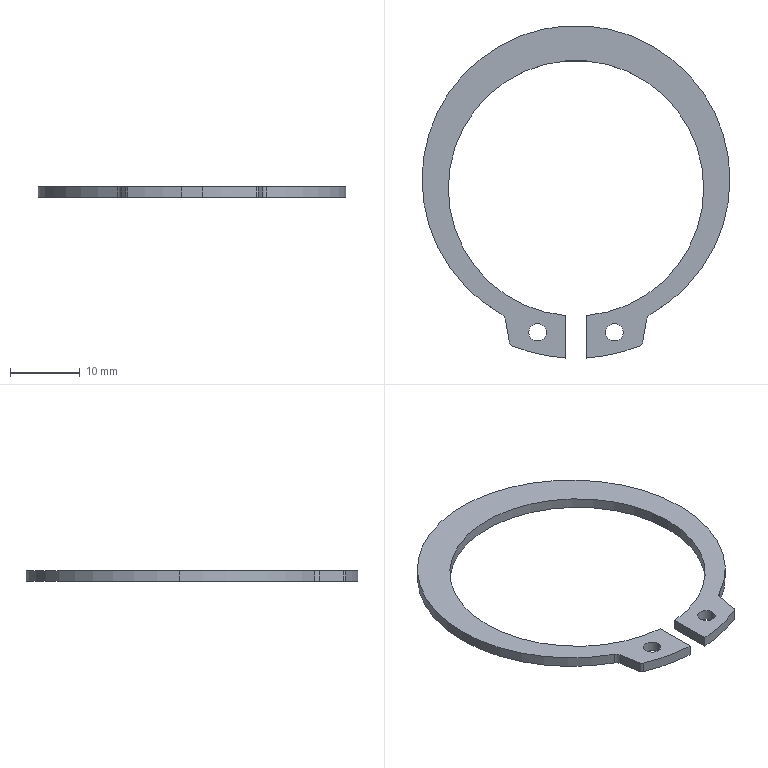Part | SolidWorks | features Extrusion 1 | 1 solid | 22 faces | box 44 x 47.504 x 1.5 mm | volume 776.12 mm3 | cylinder 16 | plane 6 | commonest cylinder face diameters 2.5 x4 36.5 x3 44 x3 1 x2 2 x2 48.6 x2
STEP:
#1=CARTESIAN_POINT('',(4.25,-21.828,0.75));
#2=VERTEX_POINT('',#1);
#3=CARTESIAN_POINT('',(6.75,-21.828,0.75));
#4=VERTEX_POINT('',#3);
#5=CARTESIAN_POINT('',(5.5,-21.828,0.75));
#6=DIRECTION('',(0.,0.,1.));
#7=DIRECTION('',(-1.,0.,0.));
#8=AXIS2_PLACEMENT_3D('',#5,#6,#7);
#9=CIRCLE('',#8,1.25);
#10=EDGE_CURVE('',#2,#4,#9,.T.);
#11=ORIENTED_EDGE('',*,*,#10,.T.);
#12=CARTESIAN_POINT('',(6.75,-21.828,-0.75));
#13=VERTEX_POINT('',#12);
#14=CARTESIAN_POINT('',(6.75,-21.828,0.75));
#15=DIRECTION('',(0.,0.,-1.));
#16=VECTOR('',#15,1000.);
#17=LINE('',#14,#16);
#18=EDGE_CURVE('',#4,#13,#17,.T.);
#19=ORIENTED_EDGE('',*,*,#18,.T.);
#20=CARTESIAN_POINT('',(4.25,-21.828,-0.75));
#21=VERTEX_POINT('',#20);
#22=CARTESIAN_POINT('',(5.5,-21.828,-0.75));
#23=DIRECTION('',(0.,0.,1.));
#24=DIRECTION('',(-1.,0.,0.));
#25=AXIS2_PLACEMENT_3D('',#22,#23,#24);
#26=CIRCLE('',#25,1.25);
#27=EDGE_CURVE('',#21,#13,#26,.T.);
#28=ORIENTED_EDGE('',*,*,#27,.F.);
#29=CARTESIAN_POINT('',(4.25,-21.828,0.75));
#30=DIRECTION('',(0.,0.,-1.));
#31=VECTOR('',#30,1000.);
#32=LINE('',#29,#31);
#33=EDGE_CURVE('',#2,#21,#32,.T.);
#34=ORIENTED_EDGE('',*,*,#33,.F.);
#35=EDGE_LOOP('',(#11,#19,#28,#34));
#36=FACE_OUTER_BOUND('',#35,.T.);
#37=CARTESIAN_POINT('',(5.5,-21.828,0.75));
#38=DIRECTION('',(0.,0.,-1.));
#39=DIRECTION('',(-1.,0.,0.));
#40=AXIS2_PLACEMENT_3D('',#37,#38,#39);
#41=CYLINDRICAL_SURFACE('',#40,1.25);
#42=ADVANCED_FACE('',(#36),#41,.F.);
#43=CARTESIAN_POINT('',(-6.75,-21.828,0.75));
#44=VERTEX_POINT('',#43);
#45=CARTESIAN_POINT('',(-4.25,-21.828,0.75));
#46=VERTEX_POINT('',#45);
#47=CARTESIAN_POINT('',(-5.5,-21.828,0.75));
#48=DIRECTION('',(0.,0.,1.));
#49=DIRECTION('',(1.,0.,0.));
#50=AXIS2_PLACEMENT_3D('',#47,#48,#49);
#51=CIRCLE('',#50,1.25);
#52=EDGE_CURVE('',#44,#46,#51,.T.);
#53=ORIENTED_EDGE('',*,*,#52,.T.);
#54=CARTESIAN_POINT('',(-4.25,-21.828,-0.75));
#55=VERTEX_POINT('',#54);
#56=CARTESIAN_POINT('',(-4.25,-21.828,0.75));
#57=DIRECTION('',(0.,0.,-1.));
#58=VECTOR('',#57,1000.);
#59=LINE('',#56,#58);
#60=EDGE_CURVE('',#46,#55,#59,.T.);
#61=ORIENTED_EDGE('',*,*,#60,.T.);
#62=CARTESIAN_POINT('',(-6.75,-21.828,-0.75));
#63=VERTEX_POINT('',#62);
#64=CARTESIAN_POINT('',(-5.5,-21.828,-0.75));
#65=DIRECTION('',(0.,0.,1.));
#66=DIRECTION('',(1.,0.,0.));
#67=AXIS2_PLACEMENT_3D('',#64,#65,#66);
#68=CIRCLE('',#67,1.25);
#69=EDGE_CURVE('',#63,#55,#68,.T.);
#70=ORIENTED_EDGE('',*,*,#69,.F.);
#71=CARTESIAN_POINT('',(-6.75,-21.828,0.75));
#72=DIRECTION('',(0.,0.,-1.));
#73=VECTOR('',#72,1000.);
#74=LINE('',#71,#73);
#75=EDGE_CURVE('',#44,#63,#74,.T.);
#76=ORIENTED_EDGE('',*,*,#75,.F.);
#77=EDGE_LOOP('',(#53,#61,#70,#76));
#78=FACE_OUTER_BOUND('',#77,.T.);
#79=CARTESIAN_POINT('',(-5.5,-21.828,0.75));
#80=DIRECTION('',(0.,0.,-1.));
#81=DIRECTION('',(-1.,0.,0.));
#82=AXIS2_PLACEMENT_3D('',#79,#80,#81);
#83=CYLINDRICAL_SURFACE('',#82,1.25);
#84=ADVANCED_FACE('',(#78),#83,.F.);
#85=CARTESIAN_POINT('',(22.,0.,0.75));
#86=VERTEX_POINT('',#85);
#87=CARTESIAN_POINT('',(-22.,0.,0.75));
#88=VERTEX_POINT('',#87);
#89=CARTESIAN_POINT('',(0.,0.,0.75));
#90=DIRECTION('',(0.,0.,1.));
#91=DIRECTION('',(1.,0.,0.));
#92=AXIS2_PLACEMENT_3D('',#89,#90,#91);
#93=CIRCLE('',#92,22.);
#94=EDGE_CURVE('',#86,#88,#93,.T.);
#95=ORIENTED_EDGE('',*,*,#94,.F.);
#96=CARTESIAN_POINT('',(22.,0.,-0.75));
#97=VERTEX_POINT('',#96);
#98=CARTESIAN_POINT('',(22.,0.,0.75));
#99=DIRECTION('',(0.,0.,-1.));
#100=VECTOR('',#99,1000.);
#101=LINE('',#98,#100);
#102=EDGE_CURVE('',#86,#97,#101,.T.);
#103=ORIENTED_EDGE('',*,*,#102,.T.);
#104=CARTESIAN_POINT('',(-22.,0.,-0.75));
#105=VERTEX_POINT('',#104);
#106=CARTESIAN_POINT('',(0.,0.,-0.75));
#107=DIRECTION('',(0.,0.,1.));
#108=DIRECTION('',(1.,0.,0.));
#109=AXIS2_PLACEMENT_3D('',#106,#107,#108);
#110=CIRCLE('',#109,22.);
#111=EDGE_CURVE('',#97,#105,#110,.T.);
#112=ORIENTED_EDGE('',*,*,#111,.T.);
#113=CARTESIAN_POINT('',(-22.,0.,0.75));
#114=DIRECTION('',(0.,0.,-1.));
#115=VECTOR('',#114,1000.);
#116=LINE('',#113,#115);
#117=EDGE_CURVE('',#88,#105,#116,.T.);
#118=ORIENTED_EDGE('',*,*,#117,.F.);
#119=EDGE_LOOP('',(#95,#103,#112,#118));
#120=FACE_OUTER_BOUND('',#119,.T.);
#121=CARTESIAN_POINT('',(0.,0.,0.75));
#122=DIRECTION('',(0.,0.,-1.));
#123=DIRECTION('',(-1.,0.,0.));
#124=AXIS2_PLACEMENT_3D('',#121,#122,#123);
#125=CYLINDRICAL_SURFACE('',#124,22.);
#126=ADVANCED_FACE('',(#120),#125,.T.);
#127=CARTESIAN_POINT('',(-10.6,-19.278,0.75));
#128=VERTEX_POINT('',#127);
#129=CARTESIAN_POINT('',(0.,0.,0.75));
#130=DIRECTION('',(0.,0.,1.));
#131=DIRECTION('',(1.,0.,0.));
#132=AXIS2_PLACEMENT_3D('',#129,#130,#131);
#133=CIRCLE('',#132,22.);
#134=EDGE_CURVE('',#88,#128,#133,.T.);
#135=ORIENTED_EDGE('',*,*,#134,.F.);
#136=ORIENTED_EDGE('',*,*,#117,.T.);
#137=CARTESIAN_POINT('',(-10.6,-19.278,-0.75));
#138=VERTEX_POINT('',#137);
#139=CARTESIAN_POINT('',(0.,0.,-0.75));
#140=DIRECTION('',(0.,0.,1.));
#141=DIRECTION('',(1.,0.,0.));
#142=AXIS2_PLACEMENT_3D('',#139,#140,#141);
#143=CIRCLE('',#142,22.);
#144=EDGE_CURVE('',#105,#138,#143,.T.);
#145=ORIENTED_EDGE('',*,*,#144,.T.);
#146=CARTESIAN_POINT('',(-10.6,-19.278,0.75));
#147=DIRECTION('',(0.,0.,-1.));
#148=VECTOR('',#147,1000.);
#149=LINE('',#146,#148);
#150=EDGE_CURVE('',#128,#138,#149,.T.);
#151=ORIENTED_EDGE('',*,*,#150,.F.);
#152=EDGE_LOOP('',(#135,#136,#145,#151));
#153=FACE_OUTER_BOUND('',#152,.T.);
#154=CARTESIAN_POINT('',(0.,0.,0.75));
#155=DIRECTION('',(0.,0.,-1.));
#156=DIRECTION('',(-1.,0.,0.));
#157=AXIS2_PLACEMENT_3D('',#154,#155,#156);
#158=CYLINDRICAL_SURFACE('',#157,22.);
#159=ADVANCED_FACE('',(#153),#158,.T.);
#160=CARTESIAN_POINT('',(18.25,-1.25,0.75));
#161=VERTEX_POINT('',#160);
#162=CARTESIAN_POINT('',(1.5,-19.438,0.75));
#163=VERTEX_POINT('',#162);
#164=CARTESIAN_POINT('',(0.,-1.25,0.75));
#165=DIRECTION('',(0.,0.,-1.));
#166=DIRECTION('',(1.,0.,0.));
#167=AXIS2_PLACEMENT_3D('',#164,#165,#166);
#168=CIRCLE('',#167,18.25);
#169=EDGE_CURVE('',#161,#163,#168,.T.);
#170=ORIENTED_EDGE('',*,*,#169,.F.);
#171=CARTESIAN_POINT('',(18.25,-1.25,-0.75));
#172=VERTEX_POINT('',#171);
#173=CARTESIAN_POINT('',(18.25,-1.25,0.75));
#174=DIRECTION('',(0.,0.,-1.));
#175=VECTOR('',#174,1000.);
#176=LINE('',#173,#175);
#177=EDGE_CURVE('',#161,#172,#176,.T.);
#178=ORIENTED_EDGE('',*,*,#177,.T.);
#179=CARTESIAN_POINT('',(1.5,-19.438,-0.75));
#180=VERTEX_POINT('',#179);
#181=CARTESIAN_POINT('',(0.,-1.25,-0.75));
#182=DIRECTION('',(0.,0.,-1.));
#183=DIRECTION('',(1.,0.,0.));
#184=AXIS2_PLACEMENT_3D('',#181,#182,#183);
#185=CIRCLE('',#184,18.25);
#186=EDGE_CURVE('',#172,#180,#185,.T.);
#187=ORIENTED_EDGE('',*,*,#186,.T.);
#188=CARTESIAN_POINT('',(1.5,-19.438,0.75));
#189=DIRECTION('',(0.,0.,-1.));
#190=VECTOR('',#189,1000.);
#191=LINE('',#188,#190);
#192=EDGE_CURVE('',#163,#180,#191,.T.);
#193=ORIENTED_EDGE('',*,*,#192,.F.);
#194=EDGE_LOOP('',(#170,#178,#187,#193));
#195=FACE_OUTER_BOUND('',#194,.T.);
#196=CARTESIAN_POINT('',(0.,-1.25,0.75));
#197=DIRECTION('',(0.,0.,-1.));
#198=DIRECTION('',(-1.,0.,0.));
#199=AXIS2_PLACEMENT_3D('',#196,#197,#198);
#200=CYLINDRICAL_SURFACE('',#199,18.25);
#201=ADVANCED_FACE('',(#195),#200,.F.);
#202=ORIENTED_EDGE('',*,*,#177,.F.);
#203=CARTESIAN_POINT('',(-18.25,-1.25,0.75));
#204=VERTEX_POINT('',#203);
#205=CARTESIAN_POINT('',(0.,-1.25,0.75));
#206=DIRECTION('',(0.,0.,-1.));
#207=DIRECTION('',(1.,0.,0.));
#208=AXIS2_PLACEMENT_3D('',#205,#206,#207);
#209=CIRCLE('',#208,18.25);
#210=EDGE_CURVE('',#204,#161,#209,.T.);
#211=ORIENTED_EDGE('',*,*,#210,.F.);
#212=CARTESIAN_POINT('',(-18.25,-1.25,-0.75));
#213=VERTEX_POINT('',#212);
#214=CARTESIAN_POINT('',(-18.25,-1.25,0.75));
#215=DIRECTION('',(0.,0.,-1.));
#216=VECTOR('',#215,1000.);
#217=LINE('',#214,#216);
#218=EDGE_CURVE('',#204,#213,#217,.T.);
#219=ORIENTED_EDGE('',*,*,#218,.T.);
#220=CARTESIAN_POINT('',(0.,-1.25,-0.75));
#221=DIRECTION('',(0.,0.,-1.));
#222=DIRECTION('',(1.,0.,0.));
#223=AXIS2_PLACEMENT_3D('',#220,#221,#222);
#224=CIRCLE('',#223,18.25);
#225=EDGE_CURVE('',#213,#172,#224,.T.);
#226=ORIENTED_EDGE('',*,*,#225,.T.);
#227=EDGE_LOOP('',(#202,#211,#219,#226));
#228=FACE_OUTER_BOUND('',#227,.T.);
#229=CARTESIAN_POINT('',(0.,-1.25,0.75));
#230=DIRECTION('',(0.,0.,-1.));
#231=DIRECTION('',(-1.,0.,0.));
#232=AXIS2_PLACEMENT_3D('',#229,#230,#231);
#233=CYLINDRICAL_SURFACE('',#232,18.25);
#234=ADVANCED_FACE('',(#228),#233,.F.);
#235=ORIENTED_EDGE('',*,*,#52,.F.);
#236=CARTESIAN_POINT('',(-5.5,-21.828,0.75));
#237=DIRECTION('',(0.,0.,1.));
#238=DIRECTION('',(1.,0.,0.));
#239=AXIS2_PLACEMENT_3D('',#236,#237,#238);
#240=CIRCLE('',#239,1.25);
#241=EDGE_CURVE('',#46,#44,#240,.T.);
#242=ORIENTED_EDGE('',*,*,#241,.F.);
#243=EDGE_LOOP('',(#235,#242));
#244=FACE_BOUND('',#243,.T.);
#245=CARTESIAN_POINT('',(-10.097,-19.981,0.75));
#246=VERTEX_POINT('',#245);
#247=CARTESIAN_POINT('',(-11.082,-20.154,0.75));
#248=DIRECTION('',(0.,0.,-1.));
#249=DIRECTION('',(1.,0.,0.));
#250=AXIS2_PLACEMENT_3D('',#247,#248,#249);
#251=CIRCLE('',#250,1.);
#252=EDGE_CURVE('',#128,#246,#251,.T.);
#253=ORIENTED_EDGE('',*,*,#252,.T.);
#254=CARTESIAN_POINT('',(-9.5,-23.366,0.75));
#255=VERTEX_POINT('',#254);
#256=CARTESIAN_POINT('',(-10.097,-19.981,0.75));
#257=DIRECTION('',(0.1736,-0.9848,0.));
#258=VECTOR('',#257,1000.);
#259=LINE('',#256,#258);
#260=EDGE_CURVE('',#246,#255,#259,.T.);
#261=ORIENTED_EDGE('',*,*,#260,.T.);
#262=CARTESIAN_POINT('',(-9.197,-23.742,0.75));
#263=VERTEX_POINT('',#262);
#264=CARTESIAN_POINT('',(-9.008,-23.28,0.75));
#265=DIRECTION('',(0.,0.,1.));
#266=DIRECTION('',(-1.,0.,0.));
#267=AXIS2_PLACEMENT_3D('',#264,#265,#266);
#268=CIRCLE('',#267,0.5);
#269=EDGE_CURVE('',#255,#263,#268,.T.);
#270=ORIENTED_EDGE('',*,*,#269,.T.);
#271=CARTESIAN_POINT('',(-1.5,-25.504,0.75));
#272=VERTEX_POINT('',#271);
#273=CARTESIAN_POINT('',(0.,-1.25,0.75));
#274=DIRECTION('',(0.,0.,1.));
#275=DIRECTION('',(-1.,0.,0.));
#276=AXIS2_PLACEMENT_3D('',#273,#274,#275);
#277=CIRCLE('',#276,24.3);
#278=EDGE_CURVE('',#263,#272,#277,.T.);
#279=ORIENTED_EDGE('',*,*,#278,.T.);
#280=CARTESIAN_POINT('',(-1.5,-19.438,0.75));
#281=VERTEX_POINT('',#280);
#282=CARTESIAN_POINT('',(-1.5,-19.438,0.75));
#283=DIRECTION('',(0.,1.,0.));
#284=VECTOR('',#283,1000.);
#285=LINE('',#282,#284);
#286=EDGE_CURVE('',#272,#281,#285,.T.);
#287=ORIENTED_EDGE('',*,*,#286,.T.);
#288=CARTESIAN_POINT('',(0.,-1.25,0.75));
#289=DIRECTION('',(0.,0.,-1.));
#290=DIRECTION('',(1.,0.,0.));
#291=AXIS2_PLACEMENT_3D('',#288,#289,#290);
#292=CIRCLE('',#291,18.25);
#293=EDGE_CURVE('',#281,#204,#292,.T.);
#294=ORIENTED_EDGE('',*,*,#293,.T.);
#295=ORIENTED_EDGE('',*,*,#210,.T.);
#296=ORIENTED_EDGE('',*,*,#169,.T.);
#297=CARTESIAN_POINT('',(1.5,-25.504,0.75));
#298=VERTEX_POINT('',#297);
#299=CARTESIAN_POINT('',(1.5,-19.438,0.75));
#300=DIRECTION('',(0.,-1.,0.));
#301=VECTOR('',#300,1000.);
#302=LINE('',#299,#301);
#303=EDGE_CURVE('',#163,#298,#302,.T.);
#304=ORIENTED_EDGE('',*,*,#303,.T.);
#305=CARTESIAN_POINT('',(9.197,-23.742,0.75));
#306=VERTEX_POINT('',#305);
#307=CARTESIAN_POINT('',(0.,-1.25,0.75));
#308=DIRECTION('',(0.,0.,1.));
#309=DIRECTION('',(1.,0.,0.));
#310=AXIS2_PLACEMENT_3D('',#307,#308,#309);
#311=CIRCLE('',#310,24.3);
#312=EDGE_CURVE('',#298,#306,#311,.T.);
#313=ORIENTED_EDGE('',*,*,#312,.T.);
#314=CARTESIAN_POINT('',(9.5,-23.366,0.75));
#315=VERTEX_POINT('',#314);
#316=CARTESIAN_POINT('',(9.008,-23.28,0.75));
#317=DIRECTION('',(0.,0.,1.));
#318=DIRECTION('',(1.,0.,0.));
#319=AXIS2_PLACEMENT_3D('',#316,#317,#318);
#320=CIRCLE('',#319,0.5);
#321=EDGE_CURVE('',#306,#315,#320,.T.);
#322=ORIENTED_EDGE('',*,*,#321,.T.);
#323=CARTESIAN_POINT('',(10.097,-19.981,0.75));
#324=VERTEX_POINT('',#323);
#325=CARTESIAN_POINT('',(10.097,-19.981,0.75));
#326=DIRECTION('',(0.1736,0.9848,0.));
#327=VECTOR('',#326,1000.);
#328=LINE('',#325,#327);
#329=EDGE_CURVE('',#315,#324,#328,.T.);
#330=ORIENTED_EDGE('',*,*,#329,.T.);
#331=CARTESIAN_POINT('',(10.6,-19.278,0.75));
#332=VERTEX_POINT('',#331);
#333=CARTESIAN_POINT('',(11.082,-20.154,0.75));
#334=DIRECTION('',(0.,0.,-1.));
#335=DIRECTION('',(-1.,0.,0.));
#336=AXIS2_PLACEMENT_3D('',#333,#334,#335);
#337=CIRCLE('',#336,1.);
#338=EDGE_CURVE('',#324,#332,#337,.T.);
#339=ORIENTED_EDGE('',*,*,#338,.T.);
#340=CARTESIAN_POINT('',(0.,0.,0.75));
#341=DIRECTION('',(0.,0.,1.));
#342=DIRECTION('',(1.,0.,0.));
#343=AXIS2_PLACEMENT_3D('',#340,#341,#342);
#344=CIRCLE('',#343,22.);
#345=EDGE_CURVE('',#332,#86,#344,.T.);
#346=ORIENTED_EDGE('',*,*,#345,.T.);
#347=ORIENTED_EDGE('',*,*,#94,.T.);
#348=ORIENTED_EDGE('',*,*,#134,.T.);
#349=EDGE_LOOP('',(#253,#261,#270,#279,#287,#294,#295,#296,#304,#313,#322,#330,#339,#346,#347,#348));
#350=FACE_OUTER_BOUND('',#349,.T.);
#351=ORIENTED_EDGE('',*,*,#10,.F.);
#352=CARTESIAN_POINT('',(5.5,-21.828,0.75));
#353=DIRECTION('',(0.,0.,1.));
#354=DIRECTION('',(-1.,0.,0.));
#355=AXIS2_PLACEMENT_3D('',#352,#353,#354);
#356=CIRCLE('',#355,1.25);
#357=EDGE_CURVE('',#4,#2,#356,.T.);
#358=ORIENTED_EDGE('',*,*,#357,.F.);
#359=EDGE_LOOP('',(#351,#358));
#360=FACE_BOUND('',#359,.T.);
#361=CARTESIAN_POINT('',(-11.082,-20.154,0.75));
#362=DIRECTION('',(0.,0.,1.));
#363=DIRECTION('',(1.,0.,0.));
#364=AXIS2_PLACEMENT_3D('',#361,#362,#363);
#365=PLANE('',#364);
#366=ADVANCED_FACE('',(#244,#350,#360),#365,.T.);
#367=ORIENTED_EDGE('',*,*,#150,.T.);
#368=CARTESIAN_POINT('',(-10.097,-19.981,-0.75));
#369=VERTEX_POINT('',#368);
#370=CARTESIAN_POINT('',(-11.082,-20.154,-0.75));
#371=DIRECTION('',(0.,0.,-1.));
#372=DIRECTION('',(1.,0.,0.));
#373=AXIS2_PLACEMENT_3D('',#370,#371,#372);
#374=CIRCLE('',#373,1.);
#375=EDGE_CURVE('',#138,#369,#374,.T.);
#376=ORIENTED_EDGE('',*,*,#375,.T.);
#377=CARTESIAN_POINT('',(-10.097,-19.981,0.75));
#378=DIRECTION('',(0.,0.,-1.));
#379=VECTOR('',#378,1000.);
#380=LINE('',#377,#379);
#381=EDGE_CURVE('',#246,#369,#380,.T.);
#382=ORIENTED_EDGE('',*,*,#381,.F.);
#383=ORIENTED_EDGE('',*,*,#252,.F.);
#384=EDGE_LOOP('',(#367,#376,#382,#383));
#385=FACE_OUTER_BOUND('',#384,.T.);
#386=CARTESIAN_POINT('',(-11.082,-20.154,0.75));
#387=DIRECTION('',(0.,0.,-1.));
#388=DIRECTION('',(-1.,0.,0.));
#389=AXIS2_PLACEMENT_3D('',#386,#387,#388);
#390=CYLINDRICAL_SURFACE('',#389,1.);
#391=ADVANCED_FACE('',(#385),#390,.F.);
#392=ORIENTED_EDGE('',*,*,#381,.T.);
#393=CARTESIAN_POINT('',(-9.5,-23.366,-0.75));
#394=VERTEX_POINT('',#393);
#395=CARTESIAN_POINT('',(-10.097,-19.981,-0.75));
#396=DIRECTION('',(0.1736,-0.9848,0.));
#397=VECTOR('',#396,1000.);
#398=LINE('',#395,#397);
#399=EDGE_CURVE('',#369,#394,#398,.T.);
#400=ORIENTED_EDGE('',*,*,#399,.T.);
#401=CARTESIAN_POINT('',(-9.5,-23.366,0.75));
#402=DIRECTION('',(0.,0.,-1.));
#403=VECTOR('',#402,1000.);
#404=LINE('',#401,#403);
#405=EDGE_CURVE('',#255,#394,#404,.T.);
#406=ORIENTED_EDGE('',*,*,#405,.F.);
#407=ORIENTED_EDGE('',*,*,#260,.F.);
#408=EDGE_LOOP('',(#392,#400,#406,#407));
#409=FACE_OUTER_BOUND('',#408,.T.);
#410=CARTESIAN_POINT('',(-10.097,-19.981,0.75));
#411=DIRECTION('',(0.9848,0.1736,0.));
#412=DIRECTION('',(-0.1736,0.9848,0.));
#413=AXIS2_PLACEMENT_3D('',#410,#411,#412);
#414=PLANE('',#413);
#415=ADVANCED_FACE('',(#409),#414,.F.);
#416=ORIENTED_EDGE('',*,*,#405,.T.);
#417=CARTESIAN_POINT('',(-9.197,-23.742,-0.75));
#418=VERTEX_POINT('',#417);
#419=CARTESIAN_POINT('',(-9.008,-23.28,-0.75));
#420=DIRECTION('',(0.,0.,1.));
#421=DIRECTION('',(-1.,0.,0.));
#422=AXIS2_PLACEMENT_3D('',#419,#420,#421);
#423=CIRCLE('',#422,0.5);
#424=EDGE_CURVE('',#394,#418,#423,.T.);
#425=ORIENTED_EDGE('',*,*,#424,.T.);
#426=CARTESIAN_POINT('',(-9.197,-23.742,0.75));
#427=DIRECTION('',(0.,0.,-1.));
#428=VECTOR('',#427,1000.);
#429=LINE('',#426,#428);
#430=EDGE_CURVE('',#263,#418,#429,.T.);
#431=ORIENTED_EDGE('',*,*,#430,.F.);
#432=ORIENTED_EDGE('',*,*,#269,.F.);
#433=EDGE_LOOP('',(#416,#425,#431,#432));
#434=FACE_OUTER_BOUND('',#433,.T.);
#435=CARTESIAN_POINT('',(-9.008,-23.28,0.75));
#436=DIRECTION('',(0.,0.,-1.));
#437=DIRECTION('',(-1.,0.,0.));
#438=AXIS2_PLACEMENT_3D('',#435,#436,#437);
#439=CYLINDRICAL_SURFACE('',#438,0.5);
#440=ADVANCED_FACE('',(#434),#439,.T.);
#441=ORIENTED_EDGE('',*,*,#430,.T.);
#442=CARTESIAN_POINT('',(-1.5,-25.504,-0.75));
#443=VERTEX_POINT('',#442);
#444=CARTESIAN_POINT('',(0.,-1.25,-0.75));
#445=DIRECTION('',(0.,0.,1.));
#446=DIRECTION('',(-1.,0.,0.));
#447=AXIS2_PLACEMENT_3D('',#444,#445,#446);
#448=CIRCLE('',#447,24.3);
#449=EDGE_CURVE('',#418,#443,#448,.T.);
#450=ORIENTED_EDGE('',*,*,#449,.T.);
#451=CARTESIAN_POINT('',(-1.5,-25.504,0.75));
#452=DIRECTION('',(0.,0.,-1.));
#453=VECTOR('',#452,1000.);
#454=LINE('',#451,#453);
#455=EDGE_CURVE('',#272,#443,#454,.T.);
#456=ORIENTED_EDGE('',*,*,#455,.F.);
#457=ORIENTED_EDGE('',*,*,#278,.F.);
#458=EDGE_LOOP('',(#441,#450,#456,#457));
#459=FACE_OUTER_BOUND('',#458,.T.);
#460=CARTESIAN_POINT('',(0.,-1.25,0.75));
#461=DIRECTION('',(0.,0.,-1.));
#462=DIRECTION('',(-1.,0.,0.));
#463=AXIS2_PLACEMENT_3D('',#460,#461,#462);
#464=CYLINDRICAL_SURFACE('',#463,24.3);
#465=ADVANCED_FACE('',(#459),#464,.T.);
#466=ORIENTED_EDGE('',*,*,#455,.T.);
#467=CARTESIAN_POINT('',(-1.5,-19.438,-0.75));
#468=VERTEX_POINT('',#467);
#469=CARTESIAN_POINT('',(-1.5,-19.438,-0.75));
#470=DIRECTION('',(0.,1.,0.));
#471=VECTOR('',#470,1000.);
#472=LINE('',#469,#471);
#473=EDGE_CURVE('',#443,#468,#472,.T.);
#474=ORIENTED_EDGE('',*,*,#473,.T.);
#475=CARTESIAN_POINT('',(-1.5,-19.438,0.75));
#476=DIRECTION('',(0.,0.,-1.));
#477=VECTOR('',#476,1000.);
#478=LINE('',#475,#477);
#479=EDGE_CURVE('',#281,#468,#478,.T.);
#480=ORIENTED_EDGE('',*,*,#479,.F.);
#481=ORIENTED_EDGE('',*,*,#286,.F.);
#482=EDGE_LOOP('',(#466,#474,#480,#481));
#483=FACE_OUTER_BOUND('',#482,.T.);
#484=CARTESIAN_POINT('',(-1.5,-19.438,0.75));
#485=DIRECTION('',(-1.,0.,0.));
#486=DIRECTION('',(0.,-1.,0.));
#487=AXIS2_PLACEMENT_3D('',#484,#485,#486);
#488=PLANE('',#487);
#489=ADVANCED_FACE('',(#483),#488,.F.);
#490=ORIENTED_EDGE('',*,*,#218,.F.);
#491=ORIENTED_EDGE('',*,*,#293,.F.);
#492=ORIENTED_EDGE('',*,*,#479,.T.);
#493=CARTESIAN_POINT('',(0.,-1.25,-0.75));
#494=DIRECTION('',(0.,0.,-1.));
#495=DIRECTION('',(1.,0.,0.));
#496=AXIS2_PLACEMENT_3D('',#493,#494,#495);
#497=CIRCLE('',#496,18.25);
#498=EDGE_CURVE('',#468,#213,#497,.T.);
#499=ORIENTED_EDGE('',*,*,#498,.T.);
#500=EDGE_LOOP('',(#490,#491,#492,#499));
#501=FACE_OUTER_BOUND('',#500,.T.);
#502=CARTESIAN_POINT('',(0.,-1.25,0.75));
#503=DIRECTION('',(0.,0.,-1.));
#504=DIRECTION('',(-1.,0.,0.));
#505=AXIS2_PLACEMENT_3D('',#502,#503,#504);
#506=CYLINDRICAL_SURFACE('',#505,18.25);
#507=ADVANCED_FACE('',(#501),#506,.F.);
#508=ORIENTED_EDGE('',*,*,#192,.T.);
#509=CARTESIAN_POINT('',(1.5,-25.504,-0.75));
#510=VERTEX_POINT('',#509);
#511=CARTESIAN_POINT('',(1.5,-19.438,-0.75));
#512=DIRECTION('',(0.,-1.,0.));
#513=VECTOR('',#512,1000.);
#514=LINE('',#511,#513);
#515=EDGE_CURVE('',#180,#510,#514,.T.);
#516=ORIENTED_EDGE('',*,*,#515,.T.);
#517=CARTESIAN_POINT('',(1.5,-25.504,0.75));
#518=DIRECTION('',(0.,0.,-1.));
#519=VECTOR('',#518,1000.);
#520=LINE('',#517,#519);
#521=EDGE_CURVE('',#298,#510,#520,.T.);
#522=ORIENTED_EDGE('',*,*,#521,.F.);
#523=ORIENTED_EDGE('',*,*,#303,.F.);
#524=EDGE_LOOP('',(#508,#516,#522,#523));
#525=FACE_OUTER_BOUND('',#524,.T.);
#526=CARTESIAN_POINT('',(1.5,-19.438,0.75));
#527=DIRECTION('',(1.,0.,0.));
#528=DIRECTION('',(0.,1.,0.));
#529=AXIS2_PLACEMENT_3D('',#526,#527,#528);
#530=PLANE('',#529);
#531=ADVANCED_FACE('',(#525),#530,.F.);
#532=ORIENTED_EDGE('',*,*,#521,.T.);
#533=CARTESIAN_POINT('',(9.197,-23.742,-0.75));
#534=VERTEX_POINT('',#533);
#535=CARTESIAN_POINT('',(0.,-1.25,-0.75));
#536=DIRECTION('',(0.,0.,1.));
#537=DIRECTION('',(1.,0.,0.));
#538=AXIS2_PLACEMENT_3D('',#535,#536,#537);
#539=CIRCLE('',#538,24.3);
#540=EDGE_CURVE('',#510,#534,#539,.T.);
#541=ORIENTED_EDGE('',*,*,#540,.T.);
#542=CARTESIAN_POINT('',(9.197,-23.742,0.75));
#543=DIRECTION('',(0.,0.,-1.));
#544=VECTOR('',#543,1000.);
#545=LINE('',#542,#544);
#546=EDGE_CURVE('',#306,#534,#545,.T.);
#547=ORIENTED_EDGE('',*,*,#546,.F.);
#548=ORIENTED_EDGE('',*,*,#312,.F.);
#549=EDGE_LOOP('',(#532,#541,#547,#548));
#550=FACE_OUTER_BOUND('',#549,.T.);
#551=CARTESIAN_POINT('',(0.,-1.25,0.75));
#552=DIRECTION('',(0.,0.,-1.));
#553=DIRECTION('',(-1.,0.,0.));
#554=AXIS2_PLACEMENT_3D('',#551,#552,#553);
#555=CYLINDRICAL_SURFACE('',#554,24.3);
#556=ADVANCED_FACE('',(#550),#555,.T.);
#557=ORIENTED_EDGE('',*,*,#546,.T.);
#558=CARTESIAN_POINT('',(9.5,-23.366,-0.75));
#559=VERTEX_POINT('',#558);
#560=CARTESIAN_POINT('',(9.008,-23.28,-0.75));
#561=DIRECTION('',(0.,0.,1.));
#562=DIRECTION('',(1.,0.,0.));
#563=AXIS2_PLACEMENT_3D('',#560,#561,#562);
#564=CIRCLE('',#563,0.5);
#565=EDGE_CURVE('',#534,#559,#564,.T.);
#566=ORIENTED_EDGE('',*,*,#565,.T.);
#567=CARTESIAN_POINT('',(9.5,-23.366,0.75));
#568=DIRECTION('',(0.,0.,-1.));
#569=VECTOR('',#568,1000.);
#570=LINE('',#567,#569);
#571=EDGE_CURVE('',#315,#559,#570,.T.);
#572=ORIENTED_EDGE('',*,*,#571,.F.);
#573=ORIENTED_EDGE('',*,*,#321,.F.);
#574=EDGE_LOOP('',(#557,#566,#572,#573));
#575=FACE_OUTER_BOUND('',#574,.T.);
#576=CARTESIAN_POINT('',(9.008,-23.28,0.75));
#577=DIRECTION('',(0.,0.,-1.));
#578=DIRECTION('',(-1.,0.,0.));
#579=AXIS2_PLACEMENT_3D('',#576,#577,#578);
#580=CYLINDRICAL_SURFACE('',#579,0.5);
#581=ADVANCED_FACE('',(#575),#580,.T.);
#582=ORIENTED_EDGE('',*,*,#571,.T.);
#583=CARTESIAN_POINT('',(10.097,-19.981,-0.75));
#584=VERTEX_POINT('',#583);
#585=CARTESIAN_POINT('',(10.097,-19.981,-0.75));
#586=DIRECTION('',(0.1736,0.9848,0.));
#587=VECTOR('',#586,1000.);
#588=LINE('',#585,#587);
#589=EDGE_CURVE('',#559,#584,#588,.T.);
#590=ORIENTED_EDGE('',*,*,#589,.T.);
#591=CARTESIAN_POINT('',(10.097,-19.981,0.75));
#592=DIRECTION('',(0.,0.,-1.));
#593=VECTOR('',#592,1000.);
#594=LINE('',#591,#593);
#595=EDGE_CURVE('',#324,#584,#594,.T.);
#596=ORIENTED_EDGE('',*,*,#595,.F.);
#597=ORIENTED_EDGE('',*,*,#329,.F.);
#598=EDGE_LOOP('',(#582,#590,#596,#597));
#599=FACE_OUTER_BOUND('',#598,.T.);
#600=CARTESIAN_POINT('',(10.097,-19.981,0.75));
#601=DIRECTION('',(-0.9848,0.1736,0.));
#602=DIRECTION('',(-0.1736,-0.9848,0.));
#603=AXIS2_PLACEMENT_3D('',#600,#601,#602);
#604=PLANE('',#603);
#605=ADVANCED_FACE('',(#599),#604,.F.);
#606=ORIENTED_EDGE('',*,*,#595,.T.);
#607=CARTESIAN_POINT('',(10.6,-19.278,-0.75));
#608=VERTEX_POINT('',#607);
#609=CARTESIAN_POINT('',(11.082,-20.154,-0.75));
#610=DIRECTION('',(0.,0.,-1.));
#611=DIRECTION('',(-1.,0.,0.));
#612=AXIS2_PLACEMENT_3D('',#609,#610,#611);
#613=CIRCLE('',#612,1.);
#614=EDGE_CURVE('',#584,#608,#613,.T.);
#615=ORIENTED_EDGE('',*,*,#614,.T.);
#616=CARTESIAN_POINT('',(10.6,-19.278,0.75));
#617=DIRECTION('',(0.,0.,-1.));
#618=VECTOR('',#617,1000.);
#619=LINE('',#616,#618);
#620=EDGE_CURVE('',#332,#608,#619,.T.);
#621=ORIENTED_EDGE('',*,*,#620,.F.);
#622=ORIENTED_EDGE('',*,*,#338,.F.);
#623=EDGE_LOOP('',(#606,#615,#621,#622));
#624=FACE_OUTER_BOUND('',#623,.T.);
#625=CARTESIAN_POINT('',(11.082,-20.154,0.75));
#626=DIRECTION('',(0.,0.,-1.));
#627=DIRECTION('',(-1.,0.,0.));
#628=AXIS2_PLACEMENT_3D('',#625,#626,#627);
#629=CYLINDRICAL_SURFACE('',#628,1.);
#630=ADVANCED_FACE('',(#624),#629,.F.);
#631=ORIENTED_EDGE('',*,*,#102,.F.);
#632=ORIENTED_EDGE('',*,*,#345,.F.);
#633=ORIENTED_EDGE('',*,*,#620,.T.);
#634=CARTESIAN_POINT('',(0.,0.,-0.75));
#635=DIRECTION('',(0.,0.,1.));
#636=DIRECTION('',(1.,0.,0.));
#637=AXIS2_PLACEMENT_3D('',#634,#635,#636);
#638=CIRCLE('',#637,22.);
#639=EDGE_CURVE('',#608,#97,#638,.T.);
#640=ORIENTED_EDGE('',*,*,#639,.T.);
#641=EDGE_LOOP('',(#631,#632,#633,#640));
#642=FACE_OUTER_BOUND('',#641,.T.);
#643=CARTESIAN_POINT('',(0.,0.,0.75));
#644=DIRECTION('',(0.,0.,-1.));
#645=DIRECTION('',(-1.,0.,0.));
#646=AXIS2_PLACEMENT_3D('',#643,#644,#645);
#647=CYLINDRICAL_SURFACE('',#646,22.);
#648=ADVANCED_FACE('',(#642),#647,.T.);
#649=ORIENTED_EDGE('',*,*,#60,.F.);
#650=ORIENTED_EDGE('',*,*,#241,.T.);
#651=ORIENTED_EDGE('',*,*,#75,.T.);
#652=CARTESIAN_POINT('',(-5.5,-21.828,-0.75));
#653=DIRECTION('',(0.,0.,1.));
#654=DIRECTION('',(1.,0.,0.));
#655=AXIS2_PLACEMENT_3D('',#652,#653,#654);
#656=CIRCLE('',#655,1.25);
#657=EDGE_CURVE('',#55,#63,#656,.T.);
#658=ORIENTED_EDGE('',*,*,#657,.F.);
#659=EDGE_LOOP('',(#649,#650,#651,#658));
#660=FACE_OUTER_BOUND('',#659,.T.);
#661=CARTESIAN_POINT('',(-5.5,-21.828,0.75));
#662=DIRECTION('',(0.,0.,-1.));
#663=DIRECTION('',(-1.,0.,0.));
#664=AXIS2_PLACEMENT_3D('',#661,#662,#663);
#665=CYLINDRICAL_SURFACE('',#664,1.25);
#666=ADVANCED_FACE('',(#660),#665,.F.);
#667=ORIENTED_EDGE('',*,*,#18,.F.);
#668=ORIENTED_EDGE('',*,*,#357,.T.);
#669=ORIENTED_EDGE('',*,*,#33,.T.);
#670=CARTESIAN_POINT('',(5.5,-21.828,-0.75));
#671=DIRECTION('',(0.,0.,1.));
#672=DIRECTION('',(-1.,0.,0.));
#673=AXIS2_PLACEMENT_3D('',#670,#671,#672);
#674=CIRCLE('',#673,1.25);
#675=EDGE_CURVE('',#13,#21,#674,.T.);
#676=ORIENTED_EDGE('',*,*,#675,.F.);
#677=EDGE_LOOP('',(#667,#668,#669,#676));
#678=FACE_OUTER_BOUND('',#677,.T.);
#679=CARTESIAN_POINT('',(5.5,-21.828,0.75));
#680=DIRECTION('',(0.,0.,-1.));
#681=DIRECTION('',(-1.,0.,0.));
#682=AXIS2_PLACEMENT_3D('',#679,#680,#681);
#683=CYLINDRICAL_SURFACE('',#682,1.25);
#684=ADVANCED_FACE('',(#678),#683,.F.);
#685=ORIENTED_EDGE('',*,*,#27,.T.);
#686=ORIENTED_EDGE('',*,*,#675,.T.);
#687=EDGE_LOOP('',(#685,#686));
#688=FACE_BOUND('',#687,.T.);
#689=ORIENTED_EDGE('',*,*,#69,.T.);
#690=ORIENTED_EDGE('',*,*,#657,.T.);
#691=EDGE_LOOP('',(#689,#690));
#692=FACE_BOUND('',#691,.T.);
#693=ORIENTED_EDGE('',*,*,#375,.F.);
#694=ORIENTED_EDGE('',*,*,#144,.F.);
#695=ORIENTED_EDGE('',*,*,#111,.F.);
#696=ORIENTED_EDGE('',*,*,#639,.F.);
#697=ORIENTED_EDGE('',*,*,#614,.F.);
#698=ORIENTED_EDGE('',*,*,#589,.F.);
#699=ORIENTED_EDGE('',*,*,#565,.F.);
#700=ORIENTED_EDGE('',*,*,#540,.F.);
#701=ORIENTED_EDGE('',*,*,#515,.F.);
#702=ORIENTED_EDGE('',*,*,#186,.F.);
#703=ORIENTED_EDGE('',*,*,#225,.F.);
#704=ORIENTED_EDGE('',*,*,#498,.F.);
#705=ORIENTED_EDGE('',*,*,#473,.F.);
#706=ORIENTED_EDGE('',*,*,#449,.F.);
#707=ORIENTED_EDGE('',*,*,#424,.F.);
#708=ORIENTED_EDGE('',*,*,#399,.F.);
#709=EDGE_LOOP('',(#693,#694,#695,#696,#697,#698,#699,#700,#701,#702,#703,#704,#705,#706,#707,#708));
#710=FACE_OUTER_BOUND('',#709,.T.);
#711=CARTESIAN_POINT('',(-11.082,-20.154,-0.75));
#712=DIRECTION('',(0.,0.,1.));
#713=DIRECTION('',(1.,0.,0.));
#714=AXIS2_PLACEMENT_3D('',#711,#712,#713);
#715=PLANE('',#714);
#716=ADVANCED_FACE('',(#688,#692,#710),#715,.F.);
#717=CLOSED_SHELL('',(#42,#84,#126,#159,#201,#234,#366,#391,#415,#440,#465,#489,#507,#531,#556,#581,#605,#630,#648,#666,#684,#716));
#718=MANIFOLD_SOLID_BREP('',#717);
#719=CARTESIAN_POINT('',(0.,0.,0.));
#720=DIRECTION('',(0.,0.,1.));
#721=DIRECTION('',(1.,0.,0.));
#722=AXIS2_PLACEMENT_3D('',#719,#720,#721);
#723=(LENGTH_UNIT()NAMED_UNIT(*)SI_UNIT(.MILLI.,.METRE.));
#724=UNCERTAINTY_MEASURE_WITH_UNIT(LENGTH_MEASURE(0.00001),#723,'','');
#725=(NAMED_UNIT(*)PLANE_ANGLE_UNIT()SI_UNIT($,.RADIAN.));
#726=(NAMED_UNIT(*)SI_UNIT($,.STERADIAN.)SOLID_ANGLE_UNIT());
#727=(GEOMETRIC_REPRESENTATION_CONTEXT(3)GLOBAL_UNCERTAINTY_ASSIGNED_CONTEXT((#724))GLOBAL_UNIT_ASSIGNED_CONTEXT((#723,#725,#726))REPRESENTATION_CONTEXT('',''));
#728=ADVANCED_BREP_SHAPE_REPRESENTATION('',(#718,#722),#727);